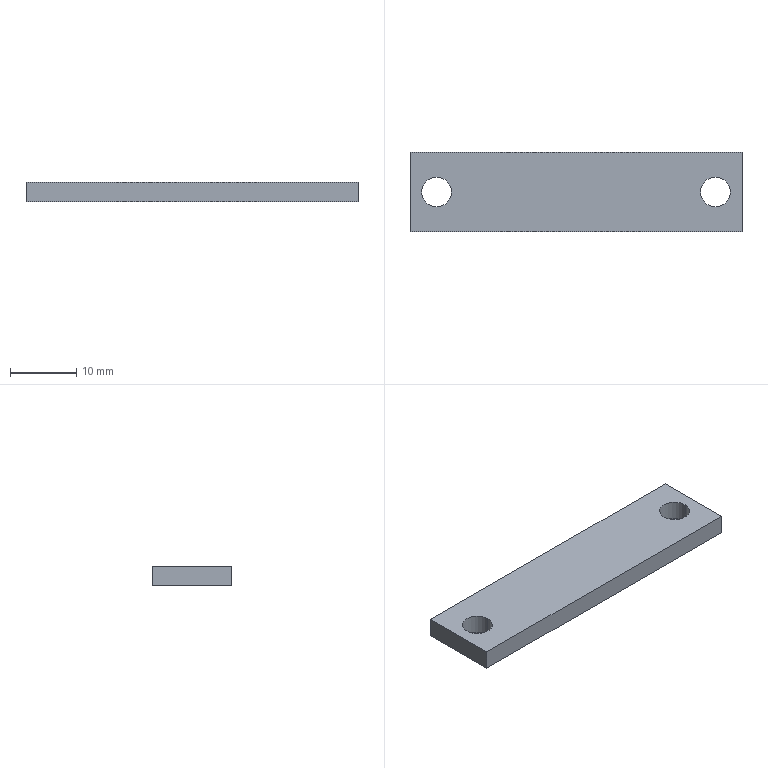Part | SolidWorks | features Extrusion 1 | 1 solid | 10 faces | box 50 x 12 x 3 mm | volume 1705 mm3 | plane 6 | cylinder 4 | commonest cylinder face diameters 4.5 x4
STEP:
#1=CARTESIAN_POINT('',(18.75,0.,1.5));
#2=VERTEX_POINT('',#1);
#3=CARTESIAN_POINT('',(23.25,0.,1.5));
#4=VERTEX_POINT('',#3);
#5=CARTESIAN_POINT('',(21.,0.,1.5));
#6=DIRECTION('',(0.,0.,1.));
#7=DIRECTION('',(1.,0.,0.));
#8=AXIS2_PLACEMENT_3D('',#5,#6,#7);
#9=CIRCLE('',#8,2.25);
#10=EDGE_CURVE('',#2,#4,#9,.T.);
#11=ORIENTED_EDGE('',*,*,#10,.T.);
#12=CARTESIAN_POINT('',(23.25,0.,-1.5));
#13=VERTEX_POINT('',#12);
#14=CARTESIAN_POINT('',(23.25,0.,1.5));
#15=DIRECTION('',(0.,0.,-1.));
#16=VECTOR('',#15,1000.);
#17=LINE('',#14,#16);
#18=EDGE_CURVE('',#4,#13,#17,.T.);
#19=ORIENTED_EDGE('',*,*,#18,.T.);
#20=CARTESIAN_POINT('',(18.75,0.,-1.5));
#21=VERTEX_POINT('',#20);
#22=CARTESIAN_POINT('',(21.,0.,-1.5));
#23=DIRECTION('',(0.,0.,1.));
#24=DIRECTION('',(1.,0.,0.));
#25=AXIS2_PLACEMENT_3D('',#22,#23,#24);
#26=CIRCLE('',#25,2.25);
#27=EDGE_CURVE('',#21,#13,#26,.T.);
#28=ORIENTED_EDGE('',*,*,#27,.F.);
#29=CARTESIAN_POINT('',(18.75,0.,1.5));
#30=DIRECTION('',(0.,0.,-1.));
#31=VECTOR('',#30,1000.);
#32=LINE('',#29,#31);
#33=EDGE_CURVE('',#2,#21,#32,.T.);
#34=ORIENTED_EDGE('',*,*,#33,.F.);
#35=EDGE_LOOP('',(#11,#19,#28,#34));
#36=FACE_OUTER_BOUND('',#35,.T.);
#37=CARTESIAN_POINT('',(21.,0.,1.5));
#38=DIRECTION('',(0.,0.,-1.));
#39=DIRECTION('',(-1.,0.,0.));
#40=AXIS2_PLACEMENT_3D('',#37,#38,#39);
#41=CYLINDRICAL_SURFACE('',#40,2.25);
#42=ADVANCED_FACE('',(#36),#41,.F.);
#43=CARTESIAN_POINT('',(-23.25,0.,1.5));
#44=VERTEX_POINT('',#43);
#45=CARTESIAN_POINT('',(-18.75,0.,1.5));
#46=VERTEX_POINT('',#45);
#47=CARTESIAN_POINT('',(-21.,0.,1.5));
#48=DIRECTION('',(0.,0.,1.));
#49=DIRECTION('',(1.,0.,0.));
#50=AXIS2_PLACEMENT_3D('',#47,#48,#49);
#51=CIRCLE('',#50,2.25);
#52=EDGE_CURVE('',#44,#46,#51,.T.);
#53=ORIENTED_EDGE('',*,*,#52,.T.);
#54=CARTESIAN_POINT('',(-18.75,0.,-1.5));
#55=VERTEX_POINT('',#54);
#56=CARTESIAN_POINT('',(-18.75,0.,1.5));
#57=DIRECTION('',(0.,0.,-1.));
#58=VECTOR('',#57,1000.);
#59=LINE('',#56,#58);
#60=EDGE_CURVE('',#46,#55,#59,.T.);
#61=ORIENTED_EDGE('',*,*,#60,.T.);
#62=CARTESIAN_POINT('',(-23.25,0.,-1.5));
#63=VERTEX_POINT('',#62);
#64=CARTESIAN_POINT('',(-21.,0.,-1.5));
#65=DIRECTION('',(0.,0.,1.));
#66=DIRECTION('',(1.,0.,0.));
#67=AXIS2_PLACEMENT_3D('',#64,#65,#66);
#68=CIRCLE('',#67,2.25);
#69=EDGE_CURVE('',#63,#55,#68,.T.);
#70=ORIENTED_EDGE('',*,*,#69,.F.);
#71=CARTESIAN_POINT('',(-23.25,0.,1.5));
#72=DIRECTION('',(0.,0.,-1.));
#73=VECTOR('',#72,1000.);
#74=LINE('',#71,#73);
#75=EDGE_CURVE('',#44,#63,#74,.T.);
#76=ORIENTED_EDGE('',*,*,#75,.F.);
#77=EDGE_LOOP('',(#53,#61,#70,#76));
#78=FACE_OUTER_BOUND('',#77,.T.);
#79=CARTESIAN_POINT('',(-21.,0.,1.5));
#80=DIRECTION('',(0.,0.,-1.));
#81=DIRECTION('',(-1.,0.,0.));
#82=AXIS2_PLACEMENT_3D('',#79,#80,#81);
#83=CYLINDRICAL_SURFACE('',#82,2.25);
#84=ADVANCED_FACE('',(#78),#83,.F.);
#85=CARTESIAN_POINT('',(25.,-6.,1.5));
#86=VERTEX_POINT('',#85);
#87=CARTESIAN_POINT('',(25.,6.,1.5));
#88=VERTEX_POINT('',#87);
#89=CARTESIAN_POINT('',(25.,-6.,1.5));
#90=DIRECTION('',(0.,1.,0.));
#91=VECTOR('',#90,1000.);
#92=LINE('',#89,#91);
#93=EDGE_CURVE('',#86,#88,#92,.T.);
#94=ORIENTED_EDGE('',*,*,#93,.T.);
#95=CARTESIAN_POINT('',(-25.,6.,1.5));
#96=VERTEX_POINT('',#95);
#97=CARTESIAN_POINT('',(-25.,6.,1.5));
#98=DIRECTION('',(-1.,0.,0.));
#99=VECTOR('',#98,1000.);
#100=LINE('',#97,#99);
#101=EDGE_CURVE('',#88,#96,#100,.T.);
#102=ORIENTED_EDGE('',*,*,#101,.T.);
#103=CARTESIAN_POINT('',(-25.,-6.,1.5));
#104=VERTEX_POINT('',#103);
#105=CARTESIAN_POINT('',(-25.,-6.,1.5));
#106=DIRECTION('',(0.,-1.,0.));
#107=VECTOR('',#106,1000.);
#108=LINE('',#105,#107);
#109=EDGE_CURVE('',#96,#104,#108,.T.);
#110=ORIENTED_EDGE('',*,*,#109,.T.);
#111=CARTESIAN_POINT('',(-25.,-6.,1.5));
#112=DIRECTION('',(1.,0.,0.));
#113=VECTOR('',#112,1000.);
#114=LINE('',#111,#113);
#115=EDGE_CURVE('',#104,#86,#114,.T.);
#116=ORIENTED_EDGE('',*,*,#115,.T.);
#117=EDGE_LOOP('',(#94,#102,#110,#116));
#118=FACE_OUTER_BOUND('',#117,.T.);
#119=ORIENTED_EDGE('',*,*,#52,.F.);
#120=CARTESIAN_POINT('',(-21.,0.,1.5));
#121=DIRECTION('',(0.,0.,1.));
#122=DIRECTION('',(1.,0.,0.));
#123=AXIS2_PLACEMENT_3D('',#120,#121,#122);
#124=CIRCLE('',#123,2.25);
#125=EDGE_CURVE('',#46,#44,#124,.T.);
#126=ORIENTED_EDGE('',*,*,#125,.F.);
#127=EDGE_LOOP('',(#119,#126));
#128=FACE_BOUND('',#127,.T.);
#129=ORIENTED_EDGE('',*,*,#10,.F.);
#130=CARTESIAN_POINT('',(21.,0.,1.5));
#131=DIRECTION('',(0.,0.,1.));
#132=DIRECTION('',(1.,0.,0.));
#133=AXIS2_PLACEMENT_3D('',#130,#131,#132);
#134=CIRCLE('',#133,2.25);
#135=EDGE_CURVE('',#4,#2,#134,.T.);
#136=ORIENTED_EDGE('',*,*,#135,.F.);
#137=EDGE_LOOP('',(#129,#136));
#138=FACE_BOUND('',#137,.T.);
#139=CARTESIAN_POINT('',(0.,0.,1.5));
#140=DIRECTION('',(0.,0.,-1.));
#141=DIRECTION('',(-1.,0.,0.));
#142=AXIS2_PLACEMENT_3D('',#139,#140,#141);
#143=PLANE('',#142);
#144=ADVANCED_FACE('',(#118,#128,#138),#143,.F.);
#145=ORIENTED_EDGE('',*,*,#69,.T.);
#146=CARTESIAN_POINT('',(-21.,0.,-1.5));
#147=DIRECTION('',(0.,0.,1.));
#148=DIRECTION('',(1.,0.,0.));
#149=AXIS2_PLACEMENT_3D('',#146,#147,#148);
#150=CIRCLE('',#149,2.25);
#151=EDGE_CURVE('',#55,#63,#150,.T.);
#152=ORIENTED_EDGE('',*,*,#151,.T.);
#153=EDGE_LOOP('',(#145,#152));
#154=FACE_BOUND('',#153,.T.);
#155=CARTESIAN_POINT('',(25.,-6.,-1.5));
#156=VERTEX_POINT('',#155);
#157=CARTESIAN_POINT('',(25.,6.,-1.5));
#158=VERTEX_POINT('',#157);
#159=CARTESIAN_POINT('',(25.,-6.,-1.5));
#160=DIRECTION('',(0.,1.,0.));
#161=VECTOR('',#160,1000.);
#162=LINE('',#159,#161);
#163=EDGE_CURVE('',#156,#158,#162,.T.);
#164=ORIENTED_EDGE('',*,*,#163,.F.);
#165=CARTESIAN_POINT('',(-25.,-6.,-1.5));
#166=VERTEX_POINT('',#165);
#167=CARTESIAN_POINT('',(-25.,-6.,-1.5));
#168=DIRECTION('',(1.,0.,0.));
#169=VECTOR('',#168,1000.);
#170=LINE('',#167,#169);
#171=EDGE_CURVE('',#166,#156,#170,.T.);
#172=ORIENTED_EDGE('',*,*,#171,.F.);
#173=CARTESIAN_POINT('',(-25.,6.,-1.5));
#174=VERTEX_POINT('',#173);
#175=CARTESIAN_POINT('',(-25.,-6.,-1.5));
#176=DIRECTION('',(0.,-1.,0.));
#177=VECTOR('',#176,1000.);
#178=LINE('',#175,#177);
#179=EDGE_CURVE('',#174,#166,#178,.T.);
#180=ORIENTED_EDGE('',*,*,#179,.F.);
#181=CARTESIAN_POINT('',(-25.,6.,-1.5));
#182=DIRECTION('',(-1.,0.,0.));
#183=VECTOR('',#182,1000.);
#184=LINE('',#181,#183);
#185=EDGE_CURVE('',#158,#174,#184,.T.);
#186=ORIENTED_EDGE('',*,*,#185,.F.);
#187=EDGE_LOOP('',(#164,#172,#180,#186));
#188=FACE_OUTER_BOUND('',#187,.T.);
#189=ORIENTED_EDGE('',*,*,#27,.T.);
#190=CARTESIAN_POINT('',(21.,0.,-1.5));
#191=DIRECTION('',(0.,0.,1.));
#192=DIRECTION('',(1.,0.,0.));
#193=AXIS2_PLACEMENT_3D('',#190,#191,#192);
#194=CIRCLE('',#193,2.25);
#195=EDGE_CURVE('',#13,#21,#194,.T.);
#196=ORIENTED_EDGE('',*,*,#195,.T.);
#197=EDGE_LOOP('',(#189,#196));
#198=FACE_BOUND('',#197,.T.);
#199=CARTESIAN_POINT('',(0.,0.,-1.5));
#200=DIRECTION('',(0.,0.,-1.));
#201=DIRECTION('',(-1.,0.,0.));
#202=AXIS2_PLACEMENT_3D('',#199,#200,#201);
#203=PLANE('',#202);
#204=ADVANCED_FACE('',(#154,#188,#198),#203,.T.);
#205=ORIENTED_EDGE('',*,*,#163,.T.);
#206=CARTESIAN_POINT('',(25.,6.,1.5));
#207=DIRECTION('',(0.,0.,-1.));
#208=VECTOR('',#207,1000.);
#209=LINE('',#206,#208);
#210=EDGE_CURVE('',#88,#158,#209,.T.);
#211=ORIENTED_EDGE('',*,*,#210,.F.);
#212=ORIENTED_EDGE('',*,*,#93,.F.);
#213=CARTESIAN_POINT('',(25.,-6.,1.5));
#214=DIRECTION('',(0.,0.,-1.));
#215=VECTOR('',#214,1000.);
#216=LINE('',#213,#215);
#217=EDGE_CURVE('',#86,#156,#216,.T.);
#218=ORIENTED_EDGE('',*,*,#217,.T.);
#219=EDGE_LOOP('',(#205,#211,#212,#218));
#220=FACE_OUTER_BOUND('',#219,.T.);
#221=CARTESIAN_POINT('',(25.,-6.,1.5));
#222=DIRECTION('',(-1.,0.,0.));
#223=DIRECTION('',(0.,0.,1.));
#224=AXIS2_PLACEMENT_3D('',#221,#222,#223);
#225=PLANE('',#224);
#226=ADVANCED_FACE('',(#220),#225,.F.);
#227=ORIENTED_EDGE('',*,*,#185,.T.);
#228=CARTESIAN_POINT('',(-25.,6.,1.5));
#229=DIRECTION('',(0.,0.,-1.));
#230=VECTOR('',#229,1000.);
#231=LINE('',#228,#230);
#232=EDGE_CURVE('',#96,#174,#231,.T.);
#233=ORIENTED_EDGE('',*,*,#232,.F.);
#234=ORIENTED_EDGE('',*,*,#101,.F.);
#235=ORIENTED_EDGE('',*,*,#210,.T.);
#236=EDGE_LOOP('',(#227,#233,#234,#235));
#237=FACE_OUTER_BOUND('',#236,.T.);
#238=CARTESIAN_POINT('',(-25.,6.,1.5));
#239=DIRECTION('',(0.,-1.,0.));
#240=DIRECTION('',(0.,0.,-1.));
#241=AXIS2_PLACEMENT_3D('',#238,#239,#240);
#242=PLANE('',#241);
#243=ADVANCED_FACE('',(#237),#242,.F.);
#244=ORIENTED_EDGE('',*,*,#179,.T.);
#245=CARTESIAN_POINT('',(-25.,-6.,1.5));
#246=DIRECTION('',(0.,0.,-1.));
#247=VECTOR('',#246,1000.);
#248=LINE('',#245,#247);
#249=EDGE_CURVE('',#104,#166,#248,.T.);
#250=ORIENTED_EDGE('',*,*,#249,.F.);
#251=ORIENTED_EDGE('',*,*,#109,.F.);
#252=ORIENTED_EDGE('',*,*,#232,.T.);
#253=EDGE_LOOP('',(#244,#250,#251,#252));
#254=FACE_OUTER_BOUND('',#253,.T.);
#255=CARTESIAN_POINT('',(-25.,-6.,1.5));
#256=DIRECTION('',(1.,0.,0.));
#257=DIRECTION('',(0.,0.,-1.));
#258=AXIS2_PLACEMENT_3D('',#255,#256,#257);
#259=PLANE('',#258);
#260=ADVANCED_FACE('',(#254),#259,.F.);
#261=ORIENTED_EDGE('',*,*,#171,.T.);
#262=ORIENTED_EDGE('',*,*,#217,.F.);
#263=ORIENTED_EDGE('',*,*,#115,.F.);
#264=ORIENTED_EDGE('',*,*,#249,.T.);
#265=EDGE_LOOP('',(#261,#262,#263,#264));
#266=FACE_OUTER_BOUND('',#265,.T.);
#267=CARTESIAN_POINT('',(-25.,-6.,1.5));
#268=DIRECTION('',(0.,1.,0.));
#269=DIRECTION('',(0.,0.,1.));
#270=AXIS2_PLACEMENT_3D('',#267,#268,#269);
#271=PLANE('',#270);
#272=ADVANCED_FACE('',(#266),#271,.F.);
#273=ORIENTED_EDGE('',*,*,#60,.F.);
#274=ORIENTED_EDGE('',*,*,#125,.T.);
#275=ORIENTED_EDGE('',*,*,#75,.T.);
#276=ORIENTED_EDGE('',*,*,#151,.F.);
#277=EDGE_LOOP('',(#273,#274,#275,#276));
#278=FACE_OUTER_BOUND('',#277,.T.);
#279=CARTESIAN_POINT('',(-21.,0.,1.5));
#280=DIRECTION('',(0.,0.,-1.));
#281=DIRECTION('',(-1.,0.,0.));
#282=AXIS2_PLACEMENT_3D('',#279,#280,#281);
#283=CYLINDRICAL_SURFACE('',#282,2.25);
#284=ADVANCED_FACE('',(#278),#283,.F.);
#285=ORIENTED_EDGE('',*,*,#18,.F.);
#286=ORIENTED_EDGE('',*,*,#135,.T.);
#287=ORIENTED_EDGE('',*,*,#33,.T.);
#288=ORIENTED_EDGE('',*,*,#195,.F.);
#289=EDGE_LOOP('',(#285,#286,#287,#288));
#290=FACE_OUTER_BOUND('',#289,.T.);
#291=CARTESIAN_POINT('',(21.,0.,1.5));
#292=DIRECTION('',(0.,0.,-1.));
#293=DIRECTION('',(-1.,0.,0.));
#294=AXIS2_PLACEMENT_3D('',#291,#292,#293);
#295=CYLINDRICAL_SURFACE('',#294,2.25);
#296=ADVANCED_FACE('',(#290),#295,.F.);
#297=CLOSED_SHELL('',(#42,#84,#144,#204,#226,#243,#260,#272,#284,#296));
#298=MANIFOLD_SOLID_BREP('',#297);
#299=CARTESIAN_POINT('',(0.,0.,0.));
#300=DIRECTION('',(0.,0.,1.));
#301=DIRECTION('',(1.,0.,0.));
#302=AXIS2_PLACEMENT_3D('',#299,#300,#301);
#303=(LENGTH_UNIT()NAMED_UNIT(*)SI_UNIT(.MILLI.,.METRE.));
#304=UNCERTAINTY_MEASURE_WITH_UNIT(LENGTH_MEASURE(0.00001),#303,'','');
#305=(NAMED_UNIT(*)PLANE_ANGLE_UNIT()SI_UNIT($,.RADIAN.));
#306=(NAMED_UNIT(*)SI_UNIT($,.STERADIAN.)SOLID_ANGLE_UNIT());
#307=(GEOMETRIC_REPRESENTATION_CONTEXT(3)GLOBAL_UNCERTAINTY_ASSIGNED_CONTEXT((#304))GLOBAL_UNIT_ASSIGNED_CONTEXT((#303,#305,#306))REPRESENTATION_CONTEXT('',''));
#308=ADVANCED_BREP_SHAPE_REPRESENTATION('',(#298,#302),#307);